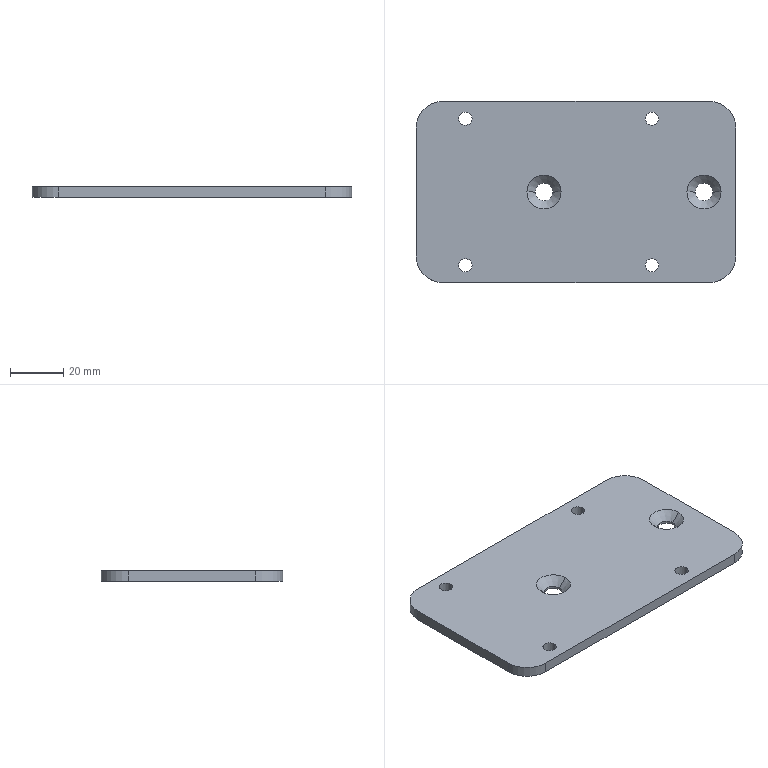Part | 1 solid | 26 faces | box 120 x 68 x 4 mm | volume 31447 mm3 | cylinder 16 | plane 6 | cone 4 | commonest cylinder face diameters 5 x8 6.6 x4 20 x4
STEP:
#1=CARTESIAN_POINT('',(-15.3,0.,0.9));
#2=VERTEX_POINT('',#1);
#3=CARTESIAN_POINT('',(-8.7,0.,0.9));
#4=VERTEX_POINT('',#3);
#5=CARTESIAN_POINT('',(-12.,0.,0.9));
#6=DIRECTION('',(0.,0.,1.));
#7=DIRECTION('',(1.,0.,0.));
#8=AXIS2_PLACEMENT_3D('',#5,#6,#7);
#9=CIRCLE('',#8,3.3);
#10=EDGE_CURVE('',#2,#4,#9,.T.);
#11=ORIENTED_EDGE('',*,*,#10,.F.);
#12=CARTESIAN_POINT('',(-18.4,0.,4.));
#13=VERTEX_POINT('',#12);
#14=CARTESIAN_POINT('',(-18.4,0.,4.));
#15=DIRECTION('',(-0.7071,0.,0.7071));
#16=VECTOR('',#15,1000.);
#17=LINE('',#14,#16);
#18=EDGE_CURVE('',#2,#13,#17,.T.);
#19=ORIENTED_EDGE('',*,*,#18,.T.);
#20=CARTESIAN_POINT('',(-5.6,0.,4.));
#21=VERTEX_POINT('',#20);
#22=CARTESIAN_POINT('',(-12.,0.,4.));
#23=DIRECTION('',(0.,0.,1.));
#24=DIRECTION('',(1.,0.,0.));
#25=AXIS2_PLACEMENT_3D('',#22,#23,#24);
#26=CIRCLE('',#25,6.4);
#27=EDGE_CURVE('',#13,#21,#26,.T.);
#28=ORIENTED_EDGE('',*,*,#27,.T.);
#29=CARTESIAN_POINT('',(-5.6,0.,4.));
#30=DIRECTION('',(0.7071,0.,0.7071));
#31=VECTOR('',#30,1000.);
#32=LINE('',#29,#31);
#33=EDGE_CURVE('',#4,#21,#32,.T.);
#34=ORIENTED_EDGE('',*,*,#33,.F.);
#35=EDGE_LOOP('',(#11,#19,#28,#34));
#36=FACE_OUTER_BOUND('',#35,.T.);
#37=CARTESIAN_POINT('',(-12.,0.,4.));
#38=DIRECTION('',(0.,0.,1.));
#39=DIRECTION('',(1.,0.,0.));
#40=AXIS2_PLACEMENT_3D('',#37,#38,#39);
#41=CONICAL_SURFACE('',#40,6.4,0.7854);
#42=ADVANCED_FACE('',(#36),#41,.F.);
#43=CARTESIAN_POINT('',(-15.3,0.,0.));
#44=VERTEX_POINT('',#43);
#45=CARTESIAN_POINT('',(-8.7,0.,0.));
#46=VERTEX_POINT('',#45);
#47=CARTESIAN_POINT('',(-12.,0.,0.));
#48=DIRECTION('',(0.,0.,1.));
#49=DIRECTION('',(1.,0.,0.));
#50=AXIS2_PLACEMENT_3D('',#47,#48,#49);
#51=CIRCLE('',#50,3.3);
#52=EDGE_CURVE('',#44,#46,#51,.T.);
#53=ORIENTED_EDGE('',*,*,#52,.F.);
#54=CARTESIAN_POINT('',(-15.3,0.,4.));
#55=DIRECTION('',(0.,0.,1.));
#56=VECTOR('',#55,1000.);
#57=LINE('',#54,#56);
#58=EDGE_CURVE('',#44,#2,#57,.T.);
#59=ORIENTED_EDGE('',*,*,#58,.T.);
#60=ORIENTED_EDGE('',*,*,#10,.T.);
#61=CARTESIAN_POINT('',(-8.7,0.,4.));
#62=DIRECTION('',(0.,0.,1.));
#63=VECTOR('',#62,1000.);
#64=LINE('',#61,#63);
#65=EDGE_CURVE('',#46,#4,#64,.T.);
#66=ORIENTED_EDGE('',*,*,#65,.F.);
#67=EDGE_LOOP('',(#53,#59,#60,#66));
#68=FACE_OUTER_BOUND('',#67,.T.);
#69=CARTESIAN_POINT('',(-12.,0.,4.));
#70=DIRECTION('',(0.,0.,1.));
#71=DIRECTION('',(1.,0.,0.));
#72=AXIS2_PLACEMENT_3D('',#69,#70,#71);
#73=CYLINDRICAL_SURFACE('',#72,3.3);
#74=ADVANCED_FACE('',(#68),#73,.F.);
#75=CARTESIAN_POINT('',(44.7,0.,0.9));
#76=VERTEX_POINT('',#75);
#77=CARTESIAN_POINT('',(51.3,0.,0.9));
#78=VERTEX_POINT('',#77);
#79=CARTESIAN_POINT('',(48.,0.,0.9));
#80=DIRECTION('',(0.,0.,1.));
#81=DIRECTION('',(1.,0.,0.));
#82=AXIS2_PLACEMENT_3D('',#79,#80,#81);
#83=CIRCLE('',#82,3.3);
#84=EDGE_CURVE('',#76,#78,#83,.T.);
#85=ORIENTED_EDGE('',*,*,#84,.F.);
#86=CARTESIAN_POINT('',(41.6,0.,4.));
#87=VERTEX_POINT('',#86);
#88=CARTESIAN_POINT('',(41.6,0.,4.));
#89=DIRECTION('',(-0.7071,0.,0.7071));
#90=VECTOR('',#89,1000.);
#91=LINE('',#88,#90);
#92=EDGE_CURVE('',#76,#87,#91,.T.);
#93=ORIENTED_EDGE('',*,*,#92,.T.);
#94=CARTESIAN_POINT('',(54.4,0.,4.));
#95=VERTEX_POINT('',#94);
#96=CARTESIAN_POINT('',(48.,0.,4.));
#97=DIRECTION('',(0.,0.,1.));
#98=DIRECTION('',(1.,0.,0.));
#99=AXIS2_PLACEMENT_3D('',#96,#97,#98);
#100=CIRCLE('',#99,6.4);
#101=EDGE_CURVE('',#87,#95,#100,.T.);
#102=ORIENTED_EDGE('',*,*,#101,.T.);
#103=CARTESIAN_POINT('',(54.4,0.,4.));
#104=DIRECTION('',(0.7071,0.,0.7071));
#105=VECTOR('',#104,1000.);
#106=LINE('',#103,#105);
#107=EDGE_CURVE('',#78,#95,#106,.T.);
#108=ORIENTED_EDGE('',*,*,#107,.F.);
#109=EDGE_LOOP('',(#85,#93,#102,#108));
#110=FACE_OUTER_BOUND('',#109,.T.);
#111=CARTESIAN_POINT('',(48.,0.,4.));
#112=DIRECTION('',(0.,0.,1.));
#113=DIRECTION('',(1.,0.,0.));
#114=AXIS2_PLACEMENT_3D('',#111,#112,#113);
#115=CONICAL_SURFACE('',#114,6.4,0.7854);
#116=ADVANCED_FACE('',(#110),#115,.F.);
#117=CARTESIAN_POINT('',(44.7,0.,0.));
#118=VERTEX_POINT('',#117);
#119=CARTESIAN_POINT('',(51.3,0.,0.));
#120=VERTEX_POINT('',#119);
#121=CARTESIAN_POINT('',(48.,0.,0.));
#122=DIRECTION('',(0.,0.,1.));
#123=DIRECTION('',(1.,0.,0.));
#124=AXIS2_PLACEMENT_3D('',#121,#122,#123);
#125=CIRCLE('',#124,3.3);
#126=EDGE_CURVE('',#118,#120,#125,.T.);
#127=ORIENTED_EDGE('',*,*,#126,.F.);
#128=CARTESIAN_POINT('',(44.7,0.,4.));
#129=DIRECTION('',(0.,0.,1.));
#130=VECTOR('',#129,1000.);
#131=LINE('',#128,#130);
#132=EDGE_CURVE('',#118,#76,#131,.T.);
#133=ORIENTED_EDGE('',*,*,#132,.T.);
#134=ORIENTED_EDGE('',*,*,#84,.T.);
#135=CARTESIAN_POINT('',(51.3,0.,4.));
#136=DIRECTION('',(0.,0.,1.));
#137=VECTOR('',#136,1000.);
#138=LINE('',#135,#137);
#139=EDGE_CURVE('',#120,#78,#138,.T.);
#140=ORIENTED_EDGE('',*,*,#139,.F.);
#141=EDGE_LOOP('',(#127,#133,#134,#140));
#142=FACE_OUTER_BOUND('',#141,.T.);
#143=CARTESIAN_POINT('',(48.,0.,4.));
#144=DIRECTION('',(0.,0.,1.));
#145=DIRECTION('',(1.,0.,0.));
#146=AXIS2_PLACEMENT_3D('',#143,#144,#145);
#147=CYLINDRICAL_SURFACE('',#146,3.3);
#148=ADVANCED_FACE('',(#142),#147,.F.);
#149=CARTESIAN_POINT('',(-44.,27.5,0.));
#150=VERTEX_POINT('',#149);
#151=CARTESIAN_POINT('',(-39.,27.5,0.));
#152=VERTEX_POINT('',#151);
#153=CARTESIAN_POINT('',(-41.5,27.5,0.));
#154=DIRECTION('',(0.,0.,1.));
#155=DIRECTION('',(1.,0.,0.));
#156=AXIS2_PLACEMENT_3D('',#153,#154,#155);
#157=CIRCLE('',#156,2.5);
#158=EDGE_CURVE('',#150,#152,#157,.T.);
#159=ORIENTED_EDGE('',*,*,#158,.F.);
#160=CARTESIAN_POINT('',(-44.,27.5,4.));
#161=VERTEX_POINT('',#160);
#162=CARTESIAN_POINT('',(-44.,27.5,4.));
#163=DIRECTION('',(0.,0.,1.));
#164=VECTOR('',#163,1000.);
#165=LINE('',#162,#164);
#166=EDGE_CURVE('',#150,#161,#165,.T.);
#167=ORIENTED_EDGE('',*,*,#166,.T.);
#168=CARTESIAN_POINT('',(-39.,27.5,4.));
#169=VERTEX_POINT('',#168);
#170=CARTESIAN_POINT('',(-41.5,27.5,4.));
#171=DIRECTION('',(0.,0.,1.));
#172=DIRECTION('',(1.,0.,0.));
#173=AXIS2_PLACEMENT_3D('',#170,#171,#172);
#174=CIRCLE('',#173,2.5);
#175=EDGE_CURVE('',#161,#169,#174,.T.);
#176=ORIENTED_EDGE('',*,*,#175,.T.);
#177=CARTESIAN_POINT('',(-39.,27.5,4.));
#178=DIRECTION('',(0.,0.,1.));
#179=VECTOR('',#178,1000.);
#180=LINE('',#177,#179);
#181=EDGE_CURVE('',#152,#169,#180,.T.);
#182=ORIENTED_EDGE('',*,*,#181,.F.);
#183=EDGE_LOOP('',(#159,#167,#176,#182));
#184=FACE_OUTER_BOUND('',#183,.T.);
#185=CARTESIAN_POINT('',(-41.5,27.5,4.));
#186=DIRECTION('',(0.,0.,1.));
#187=DIRECTION('',(1.,0.,0.));
#188=AXIS2_PLACEMENT_3D('',#185,#186,#187);
#189=CYLINDRICAL_SURFACE('',#188,2.5);
#190=ADVANCED_FACE('',(#184),#189,.F.);
#191=CARTESIAN_POINT('',(-44.,-27.5,0.));
#192=VERTEX_POINT('',#191);
#193=CARTESIAN_POINT('',(-39.,-27.5,0.));
#194=VERTEX_POINT('',#193);
#195=CARTESIAN_POINT('',(-41.5,-27.5,0.));
#196=DIRECTION('',(0.,0.,1.));
#197=DIRECTION('',(1.,0.,0.));
#198=AXIS2_PLACEMENT_3D('',#195,#196,#197);
#199=CIRCLE('',#198,2.5);
#200=EDGE_CURVE('',#192,#194,#199,.T.);
#201=ORIENTED_EDGE('',*,*,#200,.F.);
#202=CARTESIAN_POINT('',(-44.,-27.5,4.));
#203=VERTEX_POINT('',#202);
#204=CARTESIAN_POINT('',(-44.,-27.5,4.));
#205=DIRECTION('',(0.,0.,1.));
#206=VECTOR('',#205,1000.);
#207=LINE('',#204,#206);
#208=EDGE_CURVE('',#192,#203,#207,.T.);
#209=ORIENTED_EDGE('',*,*,#208,.T.);
#210=CARTESIAN_POINT('',(-39.,-27.5,4.));
#211=VERTEX_POINT('',#210);
#212=CARTESIAN_POINT('',(-41.5,-27.5,4.));
#213=DIRECTION('',(0.,0.,1.));
#214=DIRECTION('',(1.,0.,0.));
#215=AXIS2_PLACEMENT_3D('',#212,#213,#214);
#216=CIRCLE('',#215,2.5);
#217=EDGE_CURVE('',#203,#211,#216,.T.);
#218=ORIENTED_EDGE('',*,*,#217,.T.);
#219=CARTESIAN_POINT('',(-39.,-27.5,4.));
#220=DIRECTION('',(0.,0.,1.));
#221=VECTOR('',#220,1000.);
#222=LINE('',#219,#221);
#223=EDGE_CURVE('',#194,#211,#222,.T.);
#224=ORIENTED_EDGE('',*,*,#223,.F.);
#225=EDGE_LOOP('',(#201,#209,#218,#224));
#226=FACE_OUTER_BOUND('',#225,.T.);
#227=CARTESIAN_POINT('',(-41.5,-27.5,4.));
#228=DIRECTION('',(0.,0.,1.));
#229=DIRECTION('',(1.,0.,0.));
#230=AXIS2_PLACEMENT_3D('',#227,#228,#229);
#231=CYLINDRICAL_SURFACE('',#230,2.5);
#232=ADVANCED_FACE('',(#226),#231,.F.);
#233=CARTESIAN_POINT('',(26.,27.5,0.));
#234=VERTEX_POINT('',#233);
#235=CARTESIAN_POINT('',(31.,27.5,0.));
#236=VERTEX_POINT('',#235);
#237=CARTESIAN_POINT('',(28.5,27.5,0.));
#238=DIRECTION('',(0.,0.,1.));
#239=DIRECTION('',(1.,0.,0.));
#240=AXIS2_PLACEMENT_3D('',#237,#238,#239);
#241=CIRCLE('',#240,2.5);
#242=EDGE_CURVE('',#234,#236,#241,.T.);
#243=ORIENTED_EDGE('',*,*,#242,.F.);
#244=CARTESIAN_POINT('',(26.,27.5,4.));
#245=VERTEX_POINT('',#244);
#246=CARTESIAN_POINT('',(26.,27.5,4.));
#247=DIRECTION('',(0.,0.,1.));
#248=VECTOR('',#247,1000.);
#249=LINE('',#246,#248);
#250=EDGE_CURVE('',#234,#245,#249,.T.);
#251=ORIENTED_EDGE('',*,*,#250,.T.);
#252=CARTESIAN_POINT('',(31.,27.5,4.));
#253=VERTEX_POINT('',#252);
#254=CARTESIAN_POINT('',(28.5,27.5,4.));
#255=DIRECTION('',(0.,0.,1.));
#256=DIRECTION('',(1.,0.,0.));
#257=AXIS2_PLACEMENT_3D('',#254,#255,#256);
#258=CIRCLE('',#257,2.5);
#259=EDGE_CURVE('',#245,#253,#258,.T.);
#260=ORIENTED_EDGE('',*,*,#259,.T.);
#261=CARTESIAN_POINT('',(31.,27.5,4.));
#262=DIRECTION('',(0.,0.,1.));
#263=VECTOR('',#262,1000.);
#264=LINE('',#261,#263);
#265=EDGE_CURVE('',#236,#253,#264,.T.);
#266=ORIENTED_EDGE('',*,*,#265,.F.);
#267=EDGE_LOOP('',(#243,#251,#260,#266));
#268=FACE_OUTER_BOUND('',#267,.T.);
#269=CARTESIAN_POINT('',(28.5,27.5,4.));
#270=DIRECTION('',(0.,0.,1.));
#271=DIRECTION('',(1.,0.,0.));
#272=AXIS2_PLACEMENT_3D('',#269,#270,#271);
#273=CYLINDRICAL_SURFACE('',#272,2.5);
#274=ADVANCED_FACE('',(#268),#273,.F.);
#275=CARTESIAN_POINT('',(26.,-27.5,0.));
#276=VERTEX_POINT('',#275);
#277=CARTESIAN_POINT('',(31.,-27.5,0.));
#278=VERTEX_POINT('',#277);
#279=CARTESIAN_POINT('',(28.5,-27.5,0.));
#280=DIRECTION('',(0.,0.,1.));
#281=DIRECTION('',(1.,0.,0.));
#282=AXIS2_PLACEMENT_3D('',#279,#280,#281);
#283=CIRCLE('',#282,2.5);
#284=EDGE_CURVE('',#276,#278,#283,.T.);
#285=ORIENTED_EDGE('',*,*,#284,.F.);
#286=CARTESIAN_POINT('',(26.,-27.5,4.));
#287=VERTEX_POINT('',#286);
#288=CARTESIAN_POINT('',(26.,-27.5,4.));
#289=DIRECTION('',(0.,0.,1.));
#290=VECTOR('',#289,1000.);
#291=LINE('',#288,#290);
#292=EDGE_CURVE('',#276,#287,#291,.T.);
#293=ORIENTED_EDGE('',*,*,#292,.T.);
#294=CARTESIAN_POINT('',(31.,-27.5,4.));
#295=VERTEX_POINT('',#294);
#296=CARTESIAN_POINT('',(28.5,-27.5,4.));
#297=DIRECTION('',(0.,0.,1.));
#298=DIRECTION('',(1.,0.,0.));
#299=AXIS2_PLACEMENT_3D('',#296,#297,#298);
#300=CIRCLE('',#299,2.5);
#301=EDGE_CURVE('',#287,#295,#300,.T.);
#302=ORIENTED_EDGE('',*,*,#301,.T.);
#303=CARTESIAN_POINT('',(31.,-27.5,4.));
#304=DIRECTION('',(0.,0.,1.));
#305=VECTOR('',#304,1000.);
#306=LINE('',#303,#305);
#307=EDGE_CURVE('',#278,#295,#306,.T.);
#308=ORIENTED_EDGE('',*,*,#307,.F.);
#309=EDGE_LOOP('',(#285,#293,#302,#308));
#310=FACE_OUTER_BOUND('',#309,.T.);
#311=CARTESIAN_POINT('',(28.5,-27.5,4.));
#312=DIRECTION('',(0.,0.,1.));
#313=DIRECTION('',(1.,0.,0.));
#314=AXIS2_PLACEMENT_3D('',#311,#312,#313);
#315=CYLINDRICAL_SURFACE('',#314,2.5);
#316=ADVANCED_FACE('',(#310),#315,.F.);
#317=CARTESIAN_POINT('',(60.,-24.,0.));
#318=VERTEX_POINT('',#317);
#319=CARTESIAN_POINT('',(60.,24.,0.));
#320=VERTEX_POINT('',#319);
#321=CARTESIAN_POINT('',(60.,34.,0.));
#322=DIRECTION('',(0.,1.,0.));
#323=VECTOR('',#322,1000.);
#324=LINE('',#321,#323);
#325=EDGE_CURVE('',#318,#320,#324,.T.);
#326=ORIENTED_EDGE('',*,*,#325,.T.);
#327=CARTESIAN_POINT('',(60.,24.,4.));
#328=VERTEX_POINT('',#327);
#329=CARTESIAN_POINT('',(60.,24.,4.));
#330=DIRECTION('',(0.,0.,1.));
#331=VECTOR('',#330,1000.);
#332=LINE('',#329,#331);
#333=EDGE_CURVE('',#320,#328,#332,.T.);
#334=ORIENTED_EDGE('',*,*,#333,.T.);
#335=CARTESIAN_POINT('',(60.,-24.,4.));
#336=VERTEX_POINT('',#335);
#337=CARTESIAN_POINT('',(60.,34.,4.));
#338=DIRECTION('',(0.,1.,0.));
#339=VECTOR('',#338,1000.);
#340=LINE('',#337,#339);
#341=EDGE_CURVE('',#336,#328,#340,.T.);
#342=ORIENTED_EDGE('',*,*,#341,.F.);
#343=CARTESIAN_POINT('',(60.,-24.,4.));
#344=DIRECTION('',(0.,0.,-1.));
#345=VECTOR('',#344,1000.);
#346=LINE('',#343,#345);
#347=EDGE_CURVE('',#336,#318,#346,.T.);
#348=ORIENTED_EDGE('',*,*,#347,.T.);
#349=EDGE_LOOP('',(#326,#334,#342,#348));
#350=FACE_OUTER_BOUND('',#349,.T.);
#351=CARTESIAN_POINT('',(60.,34.,4.));
#352=DIRECTION('',(-1.,0.,0.));
#353=DIRECTION('',(0.,-1.,0.));
#354=AXIS2_PLACEMENT_3D('',#351,#352,#353);
#355=PLANE('',#354);
#356=ADVANCED_FACE('',(#350),#355,.F.);
#357=CARTESIAN_POINT('',(50.,34.,4.));
#358=VERTEX_POINT('',#357);
#359=CARTESIAN_POINT('',(-50.,34.,4.));
#360=VERTEX_POINT('',#359);
#361=CARTESIAN_POINT('',(-60.,34.,4.));
#362=DIRECTION('',(-1.,0.,0.));
#363=VECTOR('',#362,1000.);
#364=LINE('',#361,#363);
#365=EDGE_CURVE('',#358,#360,#364,.T.);
#366=ORIENTED_EDGE('',*,*,#365,.F.);
#367=CARTESIAN_POINT('',(50.,34.,0.));
#368=VERTEX_POINT('',#367);
#369=CARTESIAN_POINT('',(50.,34.,4.));
#370=DIRECTION('',(0.,0.,-1.));
#371=VECTOR('',#370,1000.);
#372=LINE('',#369,#371);
#373=EDGE_CURVE('',#358,#368,#372,.T.);
#374=ORIENTED_EDGE('',*,*,#373,.T.);
#375=CARTESIAN_POINT('',(-50.,34.,0.));
#376=VERTEX_POINT('',#375);
#377=CARTESIAN_POINT('',(-60.,34.,0.));
#378=DIRECTION('',(-1.,0.,0.));
#379=VECTOR('',#378,1000.);
#380=LINE('',#377,#379);
#381=EDGE_CURVE('',#368,#376,#380,.T.);
#382=ORIENTED_EDGE('',*,*,#381,.T.);
#383=CARTESIAN_POINT('',(-50.,34.,4.));
#384=DIRECTION('',(0.,0.,1.));
#385=VECTOR('',#384,1000.);
#386=LINE('',#383,#385);
#387=EDGE_CURVE('',#376,#360,#386,.T.);
#388=ORIENTED_EDGE('',*,*,#387,.T.);
#389=EDGE_LOOP('',(#366,#374,#382,#388));
#390=FACE_OUTER_BOUND('',#389,.T.);
#391=CARTESIAN_POINT('',(-60.,34.,4.));
#392=DIRECTION('',(0.,-1.,0.));
#393=DIRECTION('',(0.,0.,-1.));
#394=AXIS2_PLACEMENT_3D('',#391,#392,#393);
#395=PLANE('',#394);
#396=ADVANCED_FACE('',(#390),#395,.F.);
#397=CARTESIAN_POINT('',(-60.,24.,4.));
#398=VERTEX_POINT('',#397);
#399=CARTESIAN_POINT('',(-60.,-24.,4.));
#400=VERTEX_POINT('',#399);
#401=CARTESIAN_POINT('',(-60.,34.,4.));
#402=DIRECTION('',(0.,-1.,0.));
#403=VECTOR('',#402,1000.);
#404=LINE('',#401,#403);
#405=EDGE_CURVE('',#398,#400,#404,.T.);
#406=ORIENTED_EDGE('',*,*,#405,.F.);
#407=CARTESIAN_POINT('',(-60.,24.,0.));
#408=VERTEX_POINT('',#407);
#409=CARTESIAN_POINT('',(-60.,24.,4.));
#410=DIRECTION('',(0.,0.,-1.));
#411=VECTOR('',#410,1000.);
#412=LINE('',#409,#411);
#413=EDGE_CURVE('',#398,#408,#412,.T.);
#414=ORIENTED_EDGE('',*,*,#413,.T.);
#415=CARTESIAN_POINT('',(-60.,-24.,0.));
#416=VERTEX_POINT('',#415);
#417=CARTESIAN_POINT('',(-60.,34.,0.));
#418=DIRECTION('',(0.,-1.,0.));
#419=VECTOR('',#418,1000.);
#420=LINE('',#417,#419);
#421=EDGE_CURVE('',#408,#416,#420,.T.);
#422=ORIENTED_EDGE('',*,*,#421,.T.);
#423=CARTESIAN_POINT('',(-60.,-24.,4.));
#424=DIRECTION('',(0.,0.,1.));
#425=VECTOR('',#424,1000.);
#426=LINE('',#423,#425);
#427=EDGE_CURVE('',#416,#400,#426,.T.);
#428=ORIENTED_EDGE('',*,*,#427,.T.);
#429=EDGE_LOOP('',(#406,#414,#422,#428));
#430=FACE_OUTER_BOUND('',#429,.T.);
#431=CARTESIAN_POINT('',(-60.,34.,4.));
#432=DIRECTION('',(1.,0.,0.));
#433=DIRECTION('',(0.,0.,-1.));
#434=AXIS2_PLACEMENT_3D('',#431,#432,#433);
#435=PLANE('',#434);
#436=ADVANCED_FACE('',(#430),#435,.F.);
#437=CARTESIAN_POINT('',(-50.,-34.,0.));
#438=VERTEX_POINT('',#437);
#439=CARTESIAN_POINT('',(50.,-34.,0.));
#440=VERTEX_POINT('',#439);
#441=CARTESIAN_POINT('',(-60.,-34.,0.));
#442=DIRECTION('',(1.,0.,0.));
#443=VECTOR('',#442,1000.);
#444=LINE('',#441,#443);
#445=EDGE_CURVE('',#438,#440,#444,.T.);
#446=ORIENTED_EDGE('',*,*,#445,.T.);
#447=CARTESIAN_POINT('',(50.,-34.,4.));
#448=VERTEX_POINT('',#447);
#449=CARTESIAN_POINT('',(50.,-34.,4.));
#450=DIRECTION('',(0.,0.,1.));
#451=VECTOR('',#450,1000.);
#452=LINE('',#449,#451);
#453=EDGE_CURVE('',#440,#448,#452,.T.);
#454=ORIENTED_EDGE('',*,*,#453,.T.);
#455=CARTESIAN_POINT('',(-50.,-34.,4.));
#456=VERTEX_POINT('',#455);
#457=CARTESIAN_POINT('',(-60.,-34.,4.));
#458=DIRECTION('',(1.,0.,0.));
#459=VECTOR('',#458,1000.);
#460=LINE('',#457,#459);
#461=EDGE_CURVE('',#456,#448,#460,.T.);
#462=ORIENTED_EDGE('',*,*,#461,.F.);
#463=CARTESIAN_POINT('',(-50.,-34.,4.));
#464=DIRECTION('',(0.,0.,-1.));
#465=VECTOR('',#464,1000.);
#466=LINE('',#463,#465);
#467=EDGE_CURVE('',#456,#438,#466,.T.);
#468=ORIENTED_EDGE('',*,*,#467,.T.);
#469=EDGE_LOOP('',(#446,#454,#462,#468));
#470=FACE_OUTER_BOUND('',#469,.T.);
#471=CARTESIAN_POINT('',(-60.,-34.,4.));
#472=DIRECTION('',(0.,1.,0.));
#473=DIRECTION('',(0.,0.,1.));
#474=AXIS2_PLACEMENT_3D('',#471,#472,#473);
#475=PLANE('',#474);
#476=ADVANCED_FACE('',(#470),#475,.F.);
#477=CARTESIAN_POINT('',(-12.,0.,4.));
#478=DIRECTION('',(0.,0.,1.));
#479=DIRECTION('',(1.,0.,0.));
#480=AXIS2_PLACEMENT_3D('',#477,#478,#479);
#481=CIRCLE('',#480,6.4);
#482=EDGE_CURVE('',#21,#13,#481,.T.);
#483=ORIENTED_EDGE('',*,*,#482,.F.);
#484=ORIENTED_EDGE('',*,*,#27,.F.);
#485=EDGE_LOOP('',(#483,#484));
#486=FACE_BOUND('',#485,.T.);
#487=CARTESIAN_POINT('',(48.,0.,4.));
#488=DIRECTION('',(0.,0.,1.));
#489=DIRECTION('',(1.,0.,0.));
#490=AXIS2_PLACEMENT_3D('',#487,#488,#489);
#491=CIRCLE('',#490,6.4);
#492=EDGE_CURVE('',#95,#87,#491,.T.);
#493=ORIENTED_EDGE('',*,*,#492,.F.);
#494=ORIENTED_EDGE('',*,*,#101,.F.);
#495=EDGE_LOOP('',(#493,#494));
#496=FACE_BOUND('',#495,.T.);
#497=CARTESIAN_POINT('',(-41.5,27.5,4.));
#498=DIRECTION('',(0.,0.,1.));
#499=DIRECTION('',(1.,0.,0.));
#500=AXIS2_PLACEMENT_3D('',#497,#498,#499);
#501=CIRCLE('',#500,2.5);
#502=EDGE_CURVE('',#169,#161,#501,.T.);
#503=ORIENTED_EDGE('',*,*,#502,.F.);
#504=ORIENTED_EDGE('',*,*,#175,.F.);
#505=EDGE_LOOP('',(#503,#504));
#506=FACE_BOUND('',#505,.T.);
#507=CARTESIAN_POINT('',(-41.5,-27.5,4.));
#508=DIRECTION('',(0.,0.,1.));
#509=DIRECTION('',(1.,0.,0.));
#510=AXIS2_PLACEMENT_3D('',#507,#508,#509);
#511=CIRCLE('',#510,2.5);
#512=EDGE_CURVE('',#211,#203,#511,.T.);
#513=ORIENTED_EDGE('',*,*,#512,.F.);
#514=ORIENTED_EDGE('',*,*,#217,.F.);
#515=EDGE_LOOP('',(#513,#514));
#516=FACE_BOUND('',#515,.T.);
#517=CARTESIAN_POINT('',(28.5,27.5,4.));
#518=DIRECTION('',(0.,0.,1.));
#519=DIRECTION('',(1.,0.,0.));
#520=AXIS2_PLACEMENT_3D('',#517,#518,#519);
#521=CIRCLE('',#520,2.5);
#522=EDGE_CURVE('',#253,#245,#521,.T.);
#523=ORIENTED_EDGE('',*,*,#522,.F.);
#524=ORIENTED_EDGE('',*,*,#259,.F.);
#525=EDGE_LOOP('',(#523,#524));
#526=FACE_BOUND('',#525,.T.);
#527=CARTESIAN_POINT('',(28.5,-27.5,4.));
#528=DIRECTION('',(0.,0.,1.));
#529=DIRECTION('',(1.,0.,0.));
#530=AXIS2_PLACEMENT_3D('',#527,#528,#529);
#531=CIRCLE('',#530,2.5);
#532=EDGE_CURVE('',#295,#287,#531,.T.);
#533=ORIENTED_EDGE('',*,*,#532,.F.);
#534=ORIENTED_EDGE('',*,*,#301,.F.);
#535=EDGE_LOOP('',(#533,#534));
#536=FACE_BOUND('',#535,.T.);
#537=ORIENTED_EDGE('',*,*,#341,.T.);
#538=CARTESIAN_POINT('',(50.,24.,4.));
#539=DIRECTION('',(0.,0.,1.));
#540=DIRECTION('',(1.,0.,0.));
#541=AXIS2_PLACEMENT_3D('',#538,#539,#540);
#542=CIRCLE('',#541,10.);
#543=EDGE_CURVE('',#328,#358,#542,.T.);
#544=ORIENTED_EDGE('',*,*,#543,.T.);
#545=ORIENTED_EDGE('',*,*,#365,.T.);
#546=CARTESIAN_POINT('',(-50.,24.,4.));
#547=DIRECTION('',(0.,0.,1.));
#548=DIRECTION('',(1.,0.,0.));
#549=AXIS2_PLACEMENT_3D('',#546,#547,#548);
#550=CIRCLE('',#549,10.);
#551=EDGE_CURVE('',#360,#398,#550,.T.);
#552=ORIENTED_EDGE('',*,*,#551,.T.);
#553=ORIENTED_EDGE('',*,*,#405,.T.);
#554=CARTESIAN_POINT('',(-50.,-24.,4.));
#555=DIRECTION('',(0.,0.,1.));
#556=DIRECTION('',(1.,0.,0.));
#557=AXIS2_PLACEMENT_3D('',#554,#555,#556);
#558=CIRCLE('',#557,10.);
#559=EDGE_CURVE('',#400,#456,#558,.T.);
#560=ORIENTED_EDGE('',*,*,#559,.T.);
#561=ORIENTED_EDGE('',*,*,#461,.T.);
#562=CARTESIAN_POINT('',(50.,-24.,4.));
#563=DIRECTION('',(0.,0.,1.));
#564=DIRECTION('',(1.,0.,0.));
#565=AXIS2_PLACEMENT_3D('',#562,#563,#564);
#566=CIRCLE('',#565,10.);
#567=EDGE_CURVE('',#448,#336,#566,.T.);
#568=ORIENTED_EDGE('',*,*,#567,.T.);
#569=EDGE_LOOP('',(#537,#544,#545,#552,#553,#560,#561,#568));
#570=FACE_OUTER_BOUND('',#569,.T.);
#571=CARTESIAN_POINT('',(0.,0.,4.));
#572=DIRECTION('',(0.,0.,1.));
#573=DIRECTION('',(1.,0.,0.));
#574=AXIS2_PLACEMENT_3D('',#571,#572,#573);
#575=PLANE('',#574);
#576=ADVANCED_FACE('',(#486,#496,#506,#516,#526,#536,#570),#575,.T.);
#577=CARTESIAN_POINT('',(-12.,0.,0.));
#578=DIRECTION('',(0.,0.,1.));
#579=DIRECTION('',(1.,0.,0.));
#580=AXIS2_PLACEMENT_3D('',#577,#578,#579);
#581=CIRCLE('',#580,3.3);
#582=EDGE_CURVE('',#46,#44,#581,.T.);
#583=ORIENTED_EDGE('',*,*,#582,.T.);
#584=ORIENTED_EDGE('',*,*,#52,.T.);
#585=EDGE_LOOP('',(#583,#584));
#586=FACE_BOUND('',#585,.T.);
#587=CARTESIAN_POINT('',(48.,0.,0.));
#588=DIRECTION('',(0.,0.,1.));
#589=DIRECTION('',(1.,0.,0.));
#590=AXIS2_PLACEMENT_3D('',#587,#588,#589);
#591=CIRCLE('',#590,3.3);
#592=EDGE_CURVE('',#120,#118,#591,.T.);
#593=ORIENTED_EDGE('',*,*,#592,.T.);
#594=ORIENTED_EDGE('',*,*,#126,.T.);
#595=EDGE_LOOP('',(#593,#594));
#596=FACE_BOUND('',#595,.T.);
#597=CARTESIAN_POINT('',(-41.5,27.5,0.));
#598=DIRECTION('',(0.,0.,1.));
#599=DIRECTION('',(1.,0.,0.));
#600=AXIS2_PLACEMENT_3D('',#597,#598,#599);
#601=CIRCLE('',#600,2.5);
#602=EDGE_CURVE('',#152,#150,#601,.T.);
#603=ORIENTED_EDGE('',*,*,#602,.T.);
#604=ORIENTED_EDGE('',*,*,#158,.T.);
#605=EDGE_LOOP('',(#603,#604));
#606=FACE_BOUND('',#605,.T.);
#607=CARTESIAN_POINT('',(-41.5,-27.5,0.));
#608=DIRECTION('',(0.,0.,1.));
#609=DIRECTION('',(1.,0.,0.));
#610=AXIS2_PLACEMENT_3D('',#607,#608,#609);
#611=CIRCLE('',#610,2.5);
#612=EDGE_CURVE('',#194,#192,#611,.T.);
#613=ORIENTED_EDGE('',*,*,#612,.T.);
#614=ORIENTED_EDGE('',*,*,#200,.T.);
#615=EDGE_LOOP('',(#613,#614));
#616=FACE_BOUND('',#615,.T.);
#617=CARTESIAN_POINT('',(28.5,27.5,0.));
#618=DIRECTION('',(0.,0.,1.));
#619=DIRECTION('',(1.,0.,0.));
#620=AXIS2_PLACEMENT_3D('',#617,#618,#619);
#621=CIRCLE('',#620,2.5);
#622=EDGE_CURVE('',#236,#234,#621,.T.);
#623=ORIENTED_EDGE('',*,*,#622,.T.);
#624=ORIENTED_EDGE('',*,*,#242,.T.);
#625=EDGE_LOOP('',(#623,#624));
#626=FACE_BOUND('',#625,.T.);
#627=CARTESIAN_POINT('',(28.5,-27.5,0.));
#628=DIRECTION('',(0.,0.,1.));
#629=DIRECTION('',(1.,0.,0.));
#630=AXIS2_PLACEMENT_3D('',#627,#628,#629);
#631=CIRCLE('',#630,2.5);
#632=EDGE_CURVE('',#278,#276,#631,.T.);
#633=ORIENTED_EDGE('',*,*,#632,.T.);
#634=ORIENTED_EDGE('',*,*,#284,.T.);
#635=EDGE_LOOP('',(#633,#634));
#636=FACE_BOUND('',#635,.T.);
#637=ORIENTED_EDGE('',*,*,#381,.F.);
#638=CARTESIAN_POINT('',(50.,24.,0.));
#639=DIRECTION('',(0.,0.,-1.));
#640=DIRECTION('',(1.,0.,0.));
#641=AXIS2_PLACEMENT_3D('',#638,#639,#640);
#642=CIRCLE('',#641,10.);
#643=EDGE_CURVE('',#368,#320,#642,.T.);
#644=ORIENTED_EDGE('',*,*,#643,.T.);
#645=ORIENTED_EDGE('',*,*,#325,.F.);
#646=CARTESIAN_POINT('',(50.,-24.,0.));
#647=DIRECTION('',(0.,0.,-1.));
#648=DIRECTION('',(1.,0.,0.));
#649=AXIS2_PLACEMENT_3D('',#646,#647,#648);
#650=CIRCLE('',#649,10.);
#651=EDGE_CURVE('',#318,#440,#650,.T.);
#652=ORIENTED_EDGE('',*,*,#651,.T.);
#653=ORIENTED_EDGE('',*,*,#445,.F.);
#654=CARTESIAN_POINT('',(-50.,-24.,0.));
#655=DIRECTION('',(0.,0.,-1.));
#656=DIRECTION('',(1.,0.,0.));
#657=AXIS2_PLACEMENT_3D('',#654,#655,#656);
#658=CIRCLE('',#657,10.);
#659=EDGE_CURVE('',#438,#416,#658,.T.);
#660=ORIENTED_EDGE('',*,*,#659,.T.);
#661=ORIENTED_EDGE('',*,*,#421,.F.);
#662=CARTESIAN_POINT('',(-50.,24.,0.));
#663=DIRECTION('',(0.,0.,-1.));
#664=DIRECTION('',(1.,0.,0.));
#665=AXIS2_PLACEMENT_3D('',#662,#663,#664);
#666=CIRCLE('',#665,10.);
#667=EDGE_CURVE('',#408,#376,#666,.T.);
#668=ORIENTED_EDGE('',*,*,#667,.T.);
#669=EDGE_LOOP('',(#637,#644,#645,#652,#653,#660,#661,#668));
#670=FACE_OUTER_BOUND('',#669,.T.);
#671=CARTESIAN_POINT('',(0.,0.,0.));
#672=DIRECTION('',(0.,0.,1.));
#673=DIRECTION('',(1.,0.,0.));
#674=AXIS2_PLACEMENT_3D('',#671,#672,#673);
#675=PLANE('',#674);
#676=ADVANCED_FACE('',(#586,#596,#606,#616,#626,#636,#670),#675,.F.);
#677=ORIENTED_EDGE('',*,*,#292,.F.);
#678=ORIENTED_EDGE('',*,*,#632,.F.);
#679=ORIENTED_EDGE('',*,*,#307,.T.);
#680=ORIENTED_EDGE('',*,*,#532,.T.);
#681=EDGE_LOOP('',(#677,#678,#679,#680));
#682=FACE_OUTER_BOUND('',#681,.T.);
#683=CARTESIAN_POINT('',(28.5,-27.5,4.));
#684=DIRECTION('',(0.,0.,1.));
#685=DIRECTION('',(1.,0.,0.));
#686=AXIS2_PLACEMENT_3D('',#683,#684,#685);
#687=CYLINDRICAL_SURFACE('',#686,2.5);
#688=ADVANCED_FACE('',(#682),#687,.F.);
#689=ORIENTED_EDGE('',*,*,#250,.F.);
#690=ORIENTED_EDGE('',*,*,#622,.F.);
#691=ORIENTED_EDGE('',*,*,#265,.T.);
#692=ORIENTED_EDGE('',*,*,#522,.T.);
#693=EDGE_LOOP('',(#689,#690,#691,#692));
#694=FACE_OUTER_BOUND('',#693,.T.);
#695=CARTESIAN_POINT('',(28.5,27.5,4.));
#696=DIRECTION('',(0.,0.,1.));
#697=DIRECTION('',(1.,0.,0.));
#698=AXIS2_PLACEMENT_3D('',#695,#696,#697);
#699=CYLINDRICAL_SURFACE('',#698,2.5);
#700=ADVANCED_FACE('',(#694),#699,.F.);
#701=ORIENTED_EDGE('',*,*,#208,.F.);
#702=ORIENTED_EDGE('',*,*,#612,.F.);
#703=ORIENTED_EDGE('',*,*,#223,.T.);
#704=ORIENTED_EDGE('',*,*,#512,.T.);
#705=EDGE_LOOP('',(#701,#702,#703,#704));
#706=FACE_OUTER_BOUND('',#705,.T.);
#707=CARTESIAN_POINT('',(-41.5,-27.5,4.));
#708=DIRECTION('',(0.,0.,1.));
#709=DIRECTION('',(1.,0.,0.));
#710=AXIS2_PLACEMENT_3D('',#707,#708,#709);
#711=CYLINDRICAL_SURFACE('',#710,2.5);
#712=ADVANCED_FACE('',(#706),#711,.F.);
#713=ORIENTED_EDGE('',*,*,#166,.F.);
#714=ORIENTED_EDGE('',*,*,#602,.F.);
#715=ORIENTED_EDGE('',*,*,#181,.T.);
#716=ORIENTED_EDGE('',*,*,#502,.T.);
#717=EDGE_LOOP('',(#713,#714,#715,#716));
#718=FACE_OUTER_BOUND('',#717,.T.);
#719=CARTESIAN_POINT('',(-41.5,27.5,4.));
#720=DIRECTION('',(0.,0.,1.));
#721=DIRECTION('',(1.,0.,0.));
#722=AXIS2_PLACEMENT_3D('',#719,#720,#721);
#723=CYLINDRICAL_SURFACE('',#722,2.5);
#724=ADVANCED_FACE('',(#718),#723,.F.);
#725=ORIENTED_EDGE('',*,*,#543,.F.);
#726=ORIENTED_EDGE('',*,*,#333,.F.);
#727=ORIENTED_EDGE('',*,*,#643,.F.);
#728=ORIENTED_EDGE('',*,*,#373,.F.);
#729=EDGE_LOOP('',(#725,#726,#727,#728));
#730=FACE_OUTER_BOUND('',#729,.T.);
#731=CARTESIAN_POINT('',(50.,24.,4.));
#732=DIRECTION('',(0.,0.,-1.));
#733=DIRECTION('',(-1.,0.,0.));
#734=AXIS2_PLACEMENT_3D('',#731,#732,#733);
#735=CYLINDRICAL_SURFACE('',#734,10.);
#736=ADVANCED_FACE('',(#730),#735,.T.);
#737=ORIENTED_EDGE('',*,*,#567,.F.);
#738=ORIENTED_EDGE('',*,*,#453,.F.);
#739=ORIENTED_EDGE('',*,*,#651,.F.);
#740=ORIENTED_EDGE('',*,*,#347,.F.);
#741=EDGE_LOOP('',(#737,#738,#739,#740));
#742=FACE_OUTER_BOUND('',#741,.T.);
#743=CARTESIAN_POINT('',(50.,-24.,4.));
#744=DIRECTION('',(0.,0.,-1.));
#745=DIRECTION('',(-1.,0.,0.));
#746=AXIS2_PLACEMENT_3D('',#743,#744,#745);
#747=CYLINDRICAL_SURFACE('',#746,10.);
#748=ADVANCED_FACE('',(#742),#747,.T.);
#749=ORIENTED_EDGE('',*,*,#551,.F.);
#750=ORIENTED_EDGE('',*,*,#387,.F.);
#751=ORIENTED_EDGE('',*,*,#667,.F.);
#752=ORIENTED_EDGE('',*,*,#413,.F.);
#753=EDGE_LOOP('',(#749,#750,#751,#752));
#754=FACE_OUTER_BOUND('',#753,.T.);
#755=CARTESIAN_POINT('',(-50.,24.,4.));
#756=DIRECTION('',(0.,0.,-1.));
#757=DIRECTION('',(-1.,0.,0.));
#758=AXIS2_PLACEMENT_3D('',#755,#756,#757);
#759=CYLINDRICAL_SURFACE('',#758,10.);
#760=ADVANCED_FACE('',(#754),#759,.T.);
#761=ORIENTED_EDGE('',*,*,#559,.F.);
#762=ORIENTED_EDGE('',*,*,#427,.F.);
#763=ORIENTED_EDGE('',*,*,#659,.F.);
#764=ORIENTED_EDGE('',*,*,#467,.F.);
#765=EDGE_LOOP('',(#761,#762,#763,#764));
#766=FACE_OUTER_BOUND('',#765,.T.);
#767=CARTESIAN_POINT('',(-50.,-24.,4.));
#768=DIRECTION('',(0.,0.,-1.));
#769=DIRECTION('',(-1.,0.,0.));
#770=AXIS2_PLACEMENT_3D('',#767,#768,#769);
#771=CYLINDRICAL_SURFACE('',#770,10.);
#772=ADVANCED_FACE('',(#766),#771,.T.);
#773=ORIENTED_EDGE('',*,*,#132,.F.);
#774=ORIENTED_EDGE('',*,*,#592,.F.);
#775=ORIENTED_EDGE('',*,*,#139,.T.);
#776=CARTESIAN_POINT('',(48.,0.,0.9));
#777=DIRECTION('',(0.,0.,1.));
#778=DIRECTION('',(1.,0.,0.));
#779=AXIS2_PLACEMENT_3D('',#776,#777,#778);
#780=CIRCLE('',#779,3.3);
#781=EDGE_CURVE('',#78,#76,#780,.T.);
#782=ORIENTED_EDGE('',*,*,#781,.T.);
#783=EDGE_LOOP('',(#773,#774,#775,#782));
#784=FACE_OUTER_BOUND('',#783,.T.);
#785=CARTESIAN_POINT('',(48.,0.,4.));
#786=DIRECTION('',(0.,0.,1.));
#787=DIRECTION('',(1.,0.,0.));
#788=AXIS2_PLACEMENT_3D('',#785,#786,#787);
#789=CYLINDRICAL_SURFACE('',#788,3.3);
#790=ADVANCED_FACE('',(#784),#789,.F.);
#791=ORIENTED_EDGE('',*,*,#92,.F.);
#792=ORIENTED_EDGE('',*,*,#781,.F.);
#793=ORIENTED_EDGE('',*,*,#107,.T.);
#794=ORIENTED_EDGE('',*,*,#492,.T.);
#795=EDGE_LOOP('',(#791,#792,#793,#794));
#796=FACE_OUTER_BOUND('',#795,.T.);
#797=CARTESIAN_POINT('',(48.,0.,4.));
#798=DIRECTION('',(0.,0.,1.));
#799=DIRECTION('',(1.,0.,0.));
#800=AXIS2_PLACEMENT_3D('',#797,#798,#799);
#801=CONICAL_SURFACE('',#800,6.4,0.7854);
#802=ADVANCED_FACE('',(#796),#801,.F.);
#803=ORIENTED_EDGE('',*,*,#58,.F.);
#804=ORIENTED_EDGE('',*,*,#582,.F.);
#805=ORIENTED_EDGE('',*,*,#65,.T.);
#806=CARTESIAN_POINT('',(-12.,0.,0.9));
#807=DIRECTION('',(0.,0.,1.));
#808=DIRECTION('',(1.,0.,0.));
#809=AXIS2_PLACEMENT_3D('',#806,#807,#808);
#810=CIRCLE('',#809,3.3);
#811=EDGE_CURVE('',#4,#2,#810,.T.);
#812=ORIENTED_EDGE('',*,*,#811,.T.);
#813=EDGE_LOOP('',(#803,#804,#805,#812));
#814=FACE_OUTER_BOUND('',#813,.T.);
#815=CARTESIAN_POINT('',(-12.,0.,4.));
#816=DIRECTION('',(0.,0.,1.));
#817=DIRECTION('',(1.,0.,0.));
#818=AXIS2_PLACEMENT_3D('',#815,#816,#817);
#819=CYLINDRICAL_SURFACE('',#818,3.3);
#820=ADVANCED_FACE('',(#814),#819,.F.);
#821=ORIENTED_EDGE('',*,*,#18,.F.);
#822=ORIENTED_EDGE('',*,*,#811,.F.);
#823=ORIENTED_EDGE('',*,*,#33,.T.);
#824=ORIENTED_EDGE('',*,*,#482,.T.);
#825=EDGE_LOOP('',(#821,#822,#823,#824));
#826=FACE_OUTER_BOUND('',#825,.T.);
#827=CARTESIAN_POINT('',(-12.,0.,4.));
#828=DIRECTION('',(0.,0.,1.));
#829=DIRECTION('',(1.,0.,0.));
#830=AXIS2_PLACEMENT_3D('',#827,#828,#829);
#831=CONICAL_SURFACE('',#830,6.4,0.7854);
#832=ADVANCED_FACE('',(#826),#831,.F.);
#833=CLOSED_SHELL('',(#42,#74,#116,#148,#190,#232,#274,#316,#356,#396,#436,#476,#576,#676,#688,#700,#712,#724,#736,#748,#760,#772,#790,#802,#820,#832));
#834=MANIFOLD_SOLID_BREP('',#833);
#835=CARTESIAN_POINT('',(0.,0.,0.));
#836=DIRECTION('',(0.,0.,1.));
#837=DIRECTION('',(1.,0.,0.));
#838=AXIS2_PLACEMENT_3D('',#835,#836,#837);
#839=(LENGTH_UNIT()NAMED_UNIT(*)SI_UNIT(.MILLI.,.METRE.));
#840=UNCERTAINTY_MEASURE_WITH_UNIT(LENGTH_MEASURE(0.00001),#839,'','');
#841=(NAMED_UNIT(*)PLANE_ANGLE_UNIT()SI_UNIT($,.RADIAN.));
#842=(NAMED_UNIT(*)SI_UNIT($,.STERADIAN.)SOLID_ANGLE_UNIT());
#843=(GEOMETRIC_REPRESENTATION_CONTEXT(3)GLOBAL_UNCERTAINTY_ASSIGNED_CONTEXT((#840))GLOBAL_UNIT_ASSIGNED_CONTEXT((#839,#841,#842))REPRESENTATION_CONTEXT('',''));
#844=ADVANCED_BREP_SHAPE_REPRESENTATION('',(#834,#838),#843);